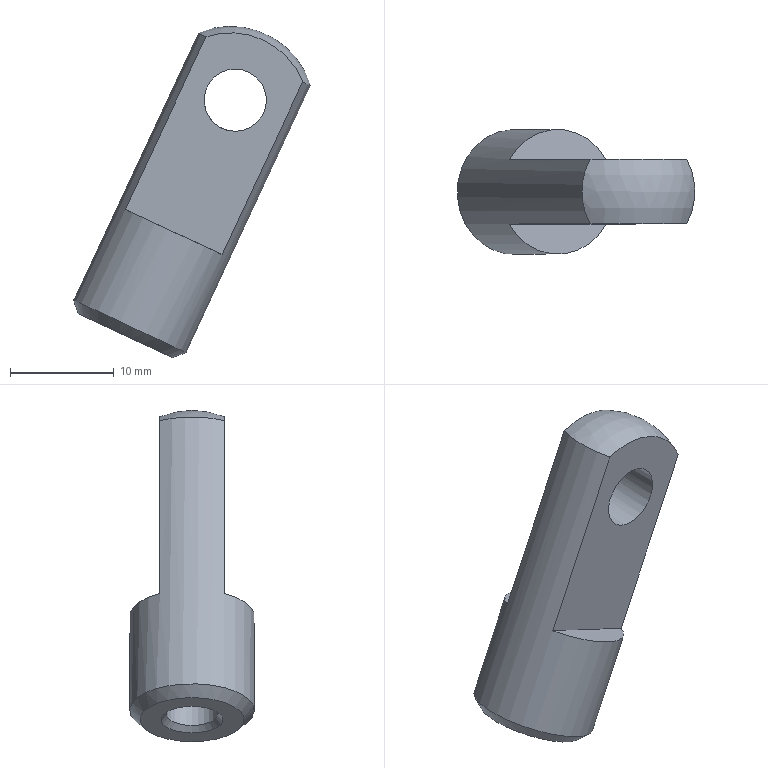Part | STEP file | 冲床-300配套压波_id678_x_t | 1 solid | 76 faces | box 22.859 x 12 x 31.872 mm | volume 2285 mm3 | plane 48 | cylinder 24 | cone 3 | sphere 1 | commonest cylinder face diameters 0.946 x5 0.757 x4 1.325 x3 1.128 x2 1.136 x2 0.568 x1